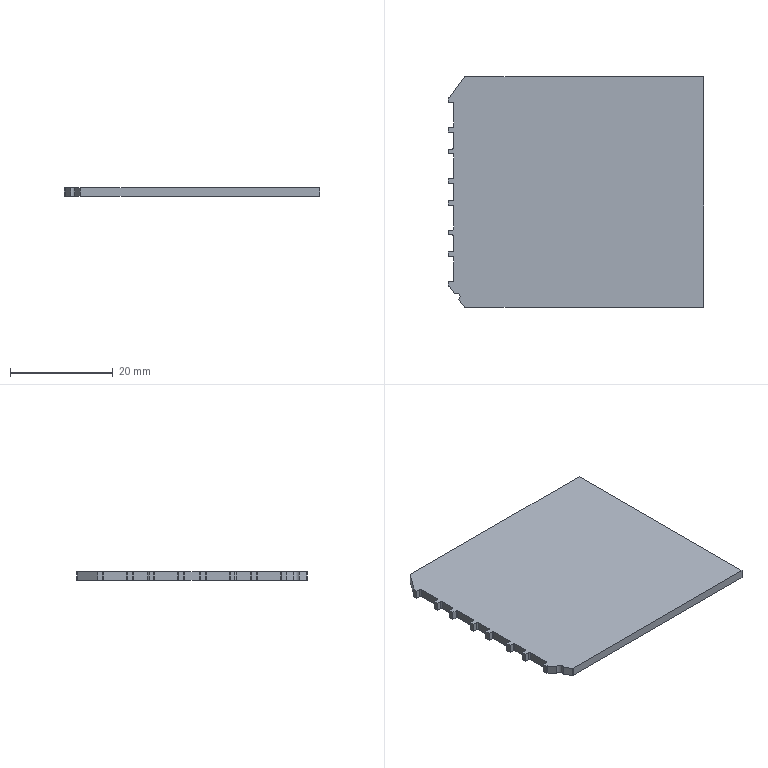Part | NX | features DATUM_CSYS 3, SKETCH 2, BLEND 1, EXTRUDE 1, HOLE PACKAGE 1, SIMPLE HOLE 1 | 1 solid | 56 faces | box 49.65 x 44.7 x 1.67 mm | volume 3632 mm3 | plane 39 | cylinder 17 | commonest cylinder face diameters 0.4 x16 1.3 x1